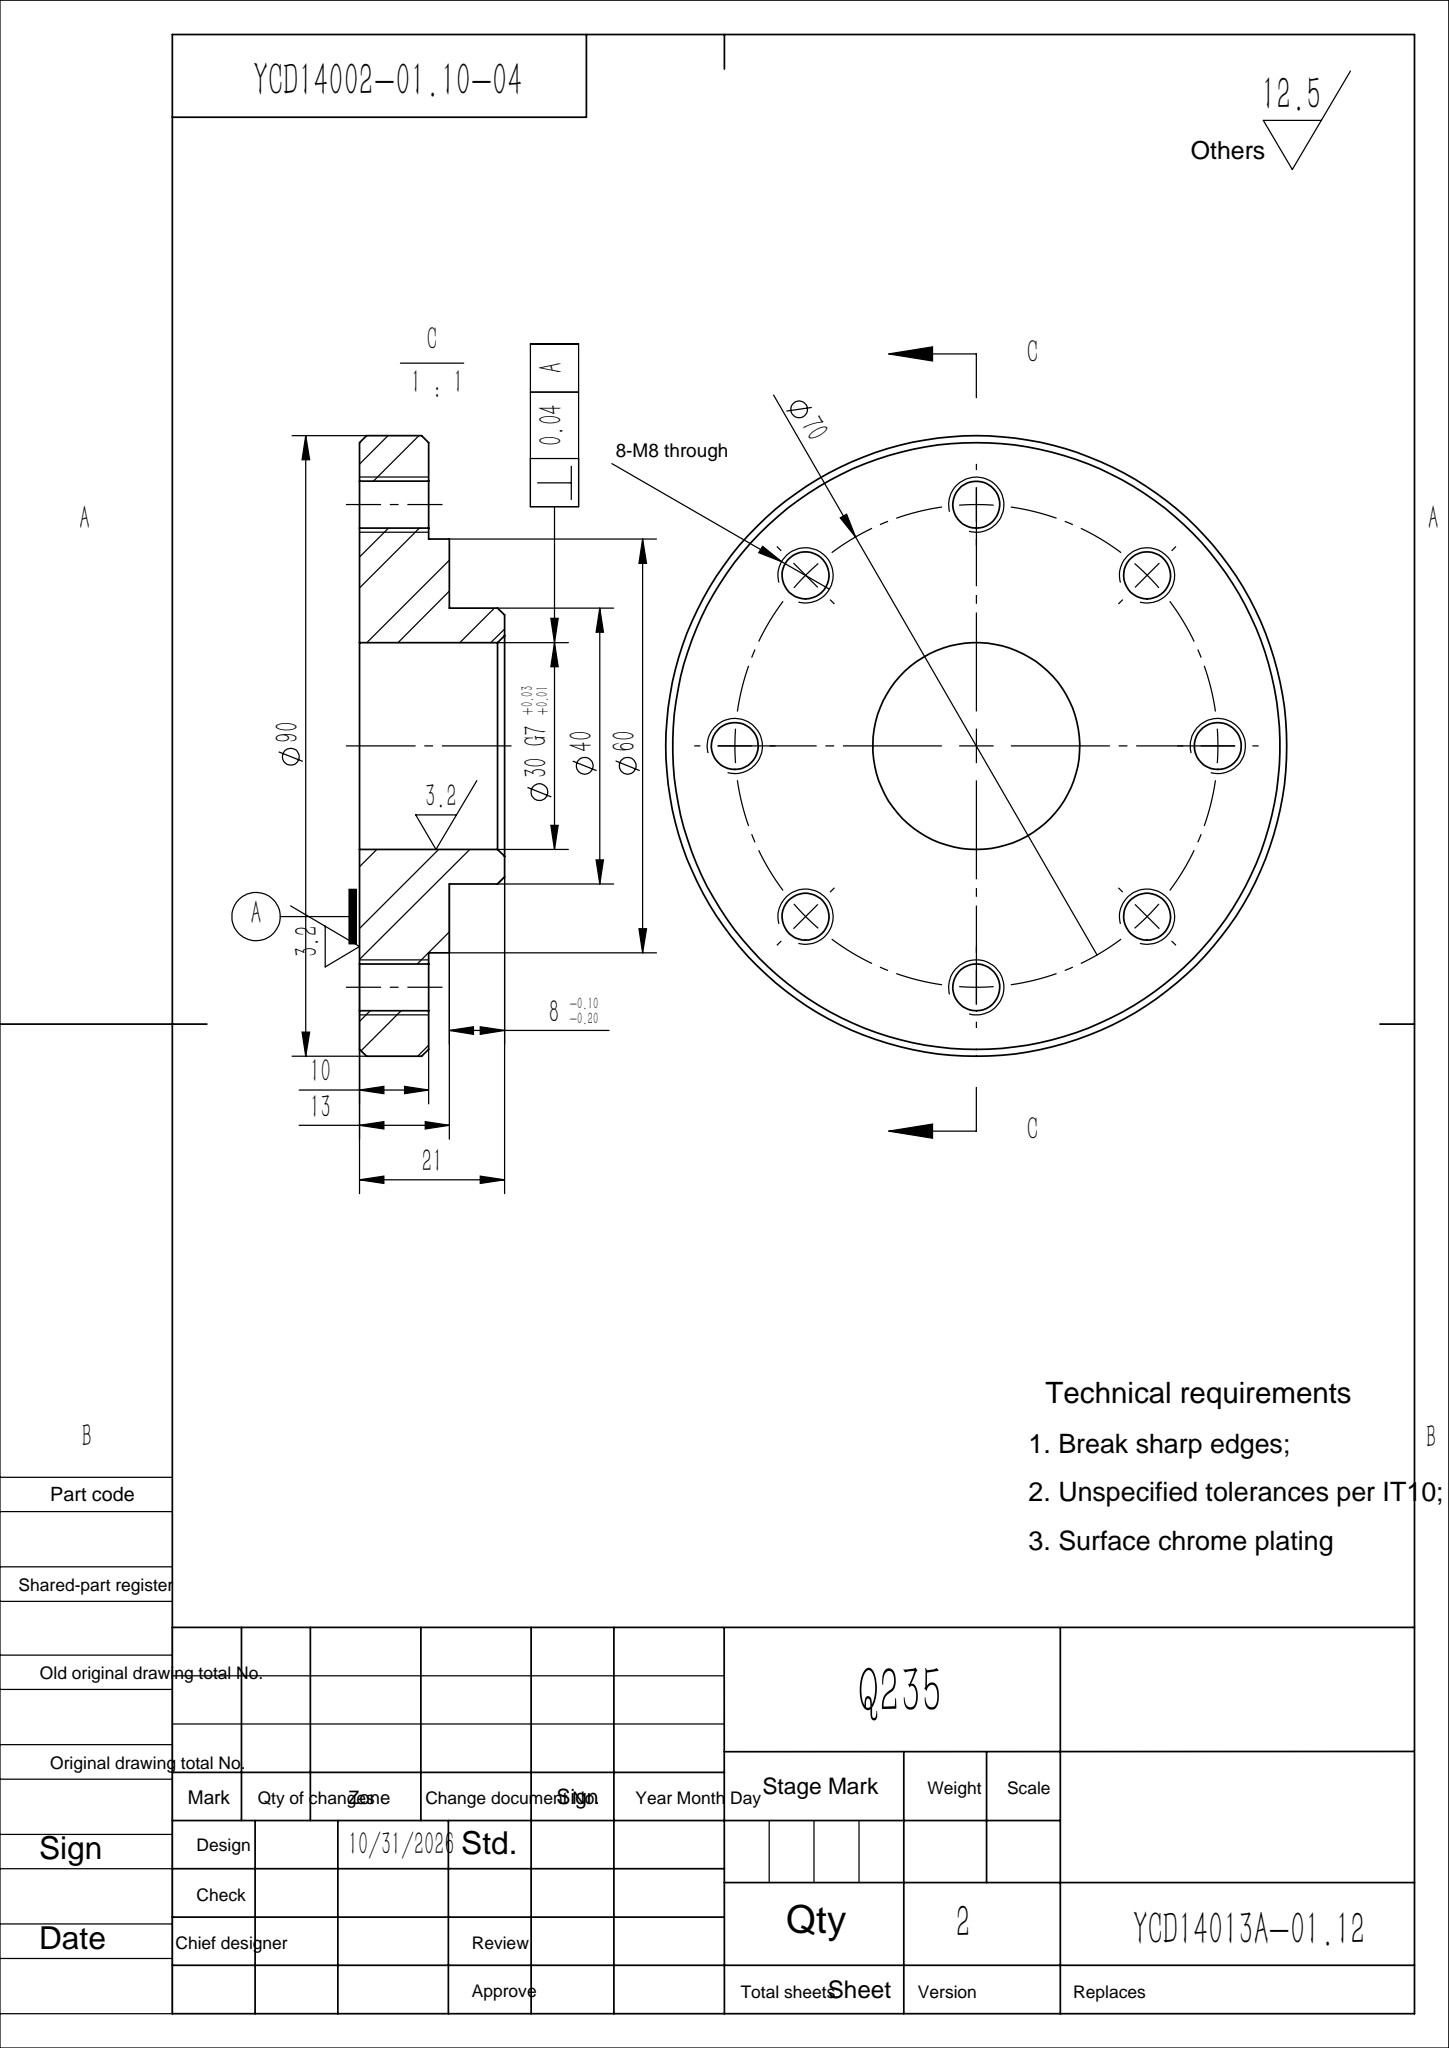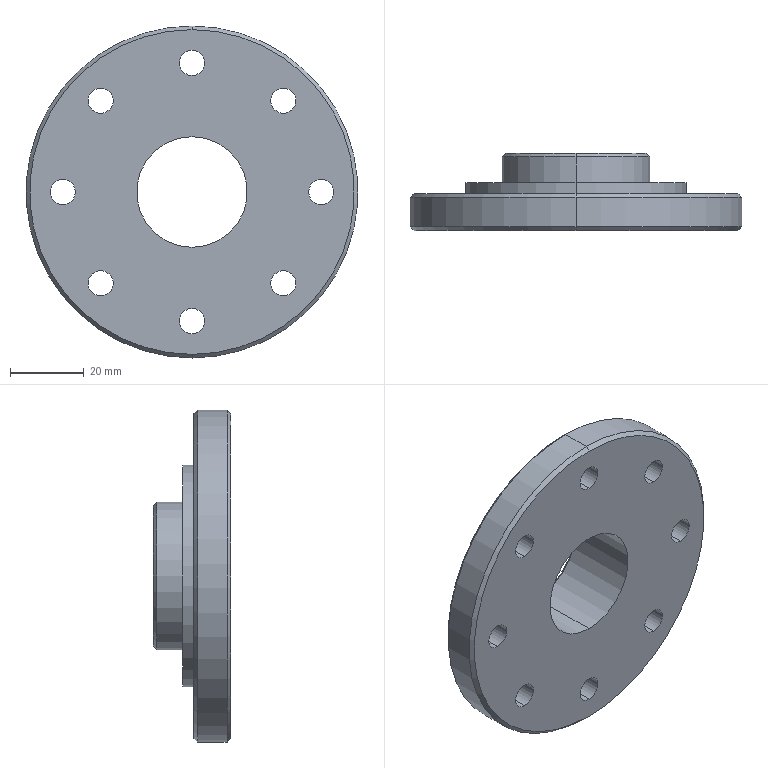Part | SolidWorks | features ICE 3, Chamfer 2, CirPattern 2, HoleWzd 2, Extrusion 1 | 1 solid | 36 faces | box 90 x 21 x 90 mm | volume 64013 mm3 | cylinder 24 | cone 8 | plane 4 | commonest cylinder face diameters 6.8 x16 30 x2 40 x2 60 x2 90 x2